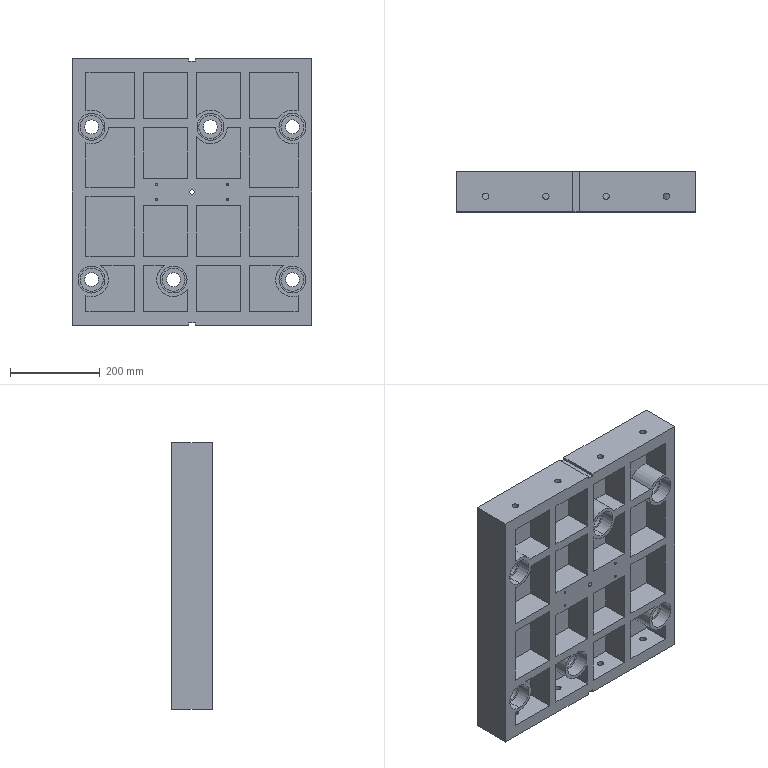Part | STEP file | LM-05-1236 | 1 solid | 237 faces | box 532 x 90 x 594 mm | volume 16985002 mm3 | plane 120 | cylinder 101 | cone 16 | commonest cylinder face diameters 14 x16 75 x15 31 x12 51.5 x12 60 x12 5 x8